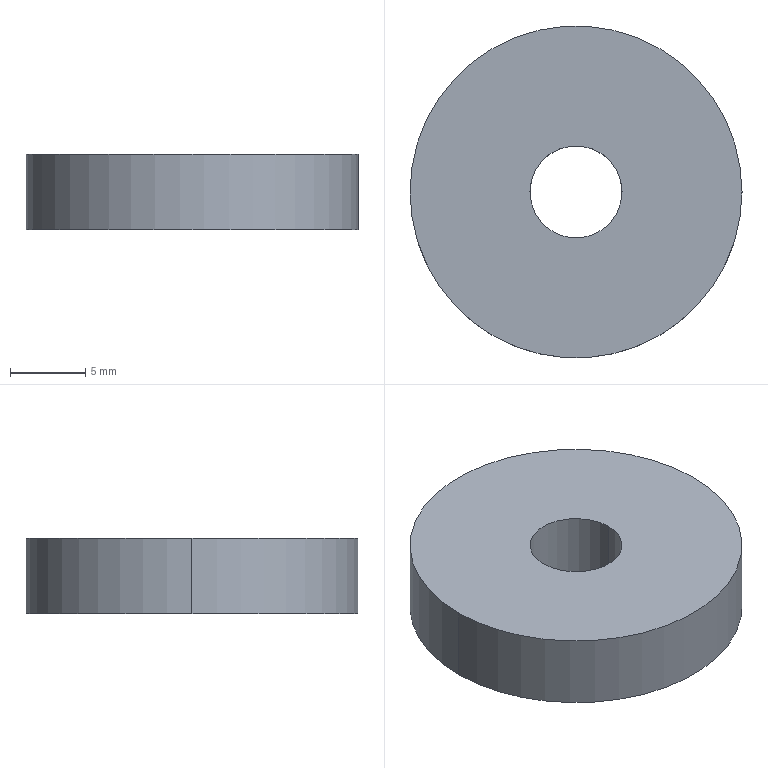Part | NX | features BREP 1 | 1 solid | 6 faces | box 22 x 22 x 5 mm | volume 1755 mm3 | cylinder 4 | plane 2 | commonest cylinder face diameters 6.1 x2 22 x2
STEP:
#1=CARTESIAN_POINT('',(3.05,0.,5.));
#2=VERTEX_POINT('',#1);
#3=CARTESIAN_POINT('',(3.05,0.,0.));
#4=VERTEX_POINT('',#3);
#5=CARTESIAN_POINT('',(3.05,0.,5.));
#6=DIRECTION('',(0.,0.,-1.));
#7=VECTOR('',#6,1000.);
#8=LINE('',#5,#7);
#9=EDGE_CURVE('',#2,#4,#8,.T.);
#10=ORIENTED_EDGE('',*,*,#9,.F.);
#11=CARTESIAN_POINT('',(-3.05,0.,5.));
#12=VERTEX_POINT('',#11);
#13=CARTESIAN_POINT('',(0.,0.,5.));
#14=DIRECTION('',(0.,0.,1.));
#15=DIRECTION('',(1.,0.,0.));
#16=AXIS2_PLACEMENT_3D('',#13,#14,#15);
#17=CIRCLE('',#16,3.05);
#18=EDGE_CURVE('',#2,#12,#17,.T.);
#19=ORIENTED_EDGE('',*,*,#18,.T.);
#20=CARTESIAN_POINT('',(-3.05,0.,0.));
#21=VERTEX_POINT('',#20);
#22=CARTESIAN_POINT('',(-3.05,0.,5.));
#23=DIRECTION('',(0.,0.,-1.));
#24=VECTOR('',#23,1000.);
#25=LINE('',#22,#24);
#26=EDGE_CURVE('',#12,#21,#25,.T.);
#27=ORIENTED_EDGE('',*,*,#26,.T.);
#28=CARTESIAN_POINT('',(0.,0.,0.));
#29=DIRECTION('',(0.,0.,1.));
#30=DIRECTION('',(1.,0.,0.));
#31=AXIS2_PLACEMENT_3D('',#28,#29,#30);
#32=CIRCLE('',#31,3.05);
#33=EDGE_CURVE('',#4,#21,#32,.T.);
#34=ORIENTED_EDGE('',*,*,#33,.F.);
#35=EDGE_LOOP('',(#10,#19,#27,#34));
#36=FACE_BOUND('',#35,.T.);
#37=CARTESIAN_POINT('',(0.,0.,5.));
#38=DIRECTION('',(0.,0.,-1.));
#39=DIRECTION('',(-1.,0.,0.));
#40=AXIS2_PLACEMENT_3D('',#37,#38,#39);
#41=CYLINDRICAL_SURFACE('',#40,3.05);
#42=ADVANCED_FACE('',(#36),#41,.F.);
#43=CARTESIAN_POINT('',(11.,0.,5.));
#44=VERTEX_POINT('',#43);
#45=CARTESIAN_POINT('',(11.,0.,0.));
#46=VERTEX_POINT('',#45);
#47=CARTESIAN_POINT('',(11.,0.,5.));
#48=DIRECTION('',(0.,0.,-1.));
#49=VECTOR('',#48,1000.);
#50=LINE('',#47,#49);
#51=EDGE_CURVE('',#44,#46,#50,.T.);
#52=ORIENTED_EDGE('',*,*,#51,.F.);
#53=CARTESIAN_POINT('',(-11.,0.,5.));
#54=VERTEX_POINT('',#53);
#55=CARTESIAN_POINT('',(0.,0.,5.));
#56=DIRECTION('',(0.,0.,1.));
#57=DIRECTION('',(1.,0.,0.));
#58=AXIS2_PLACEMENT_3D('',#55,#56,#57);
#59=CIRCLE('',#58,11.);
#60=EDGE_CURVE('',#54,#44,#59,.T.);
#61=ORIENTED_EDGE('',*,*,#60,.F.);
#62=CARTESIAN_POINT('',(-11.,0.,0.));
#63=VERTEX_POINT('',#62);
#64=CARTESIAN_POINT('',(-11.,0.,5.));
#65=DIRECTION('',(0.,0.,-1.));
#66=VECTOR('',#65,1000.);
#67=LINE('',#64,#66);
#68=EDGE_CURVE('',#54,#63,#67,.T.);
#69=ORIENTED_EDGE('',*,*,#68,.T.);
#70=CARTESIAN_POINT('',(0.,0.,0.));
#71=DIRECTION('',(0.,0.,1.));
#72=DIRECTION('',(1.,0.,0.));
#73=AXIS2_PLACEMENT_3D('',#70,#71,#72);
#74=CIRCLE('',#73,11.);
#75=EDGE_CURVE('',#63,#46,#74,.T.);
#76=ORIENTED_EDGE('',*,*,#75,.T.);
#77=EDGE_LOOP('',(#52,#61,#69,#76));
#78=FACE_BOUND('',#77,.T.);
#79=CARTESIAN_POINT('',(0.,0.,5.));
#80=DIRECTION('',(0.,0.,-1.));
#81=DIRECTION('',(-1.,0.,0.));
#82=AXIS2_PLACEMENT_3D('',#79,#80,#81);
#83=CYLINDRICAL_SURFACE('',#82,11.);
#84=ADVANCED_FACE('',(#78),#83,.T.);
#85=CARTESIAN_POINT('',(0.,0.,0.));
#86=DIRECTION('',(0.,0.,1.));
#87=DIRECTION('',(1.,0.,0.));
#88=AXIS2_PLACEMENT_3D('',#85,#86,#87);
#89=CIRCLE('',#88,3.05);
#90=EDGE_CURVE('',#21,#4,#89,.T.);
#91=ORIENTED_EDGE('',*,*,#90,.T.);
#92=ORIENTED_EDGE('',*,*,#33,.T.);
#93=EDGE_LOOP('',(#91,#92));
#94=FACE_BOUND('',#93,.T.);
#95=ORIENTED_EDGE('',*,*,#75,.F.);
#96=CARTESIAN_POINT('',(0.,0.,0.));
#97=DIRECTION('',(0.,0.,1.));
#98=DIRECTION('',(1.,0.,0.));
#99=AXIS2_PLACEMENT_3D('',#96,#97,#98);
#100=CIRCLE('',#99,11.);
#101=EDGE_CURVE('',#46,#63,#100,.T.);
#102=ORIENTED_EDGE('',*,*,#101,.F.);
#103=EDGE_LOOP('',(#95,#102));
#104=FACE_BOUND('',#103,.T.);
#105=CARTESIAN_POINT('',(0.,0.,0.));
#106=DIRECTION('',(0.,0.,1.));
#107=DIRECTION('',(1.,0.,0.));
#108=AXIS2_PLACEMENT_3D('',#105,#106,#107);
#109=PLANE('',#108);
#110=ADVANCED_FACE('',(#94,#104),#109,.F.);
#111=CARTESIAN_POINT('',(0.,0.,5.));
#112=DIRECTION('',(0.,0.,1.));
#113=DIRECTION('',(1.,0.,0.));
#114=AXIS2_PLACEMENT_3D('',#111,#112,#113);
#115=CIRCLE('',#114,3.05);
#116=EDGE_CURVE('',#12,#2,#115,.T.);
#117=ORIENTED_EDGE('',*,*,#116,.F.);
#118=ORIENTED_EDGE('',*,*,#18,.F.);
#119=EDGE_LOOP('',(#117,#118));
#120=FACE_BOUND('',#119,.T.);
#121=ORIENTED_EDGE('',*,*,#60,.T.);
#122=CARTESIAN_POINT('',(0.,0.,5.));
#123=DIRECTION('',(0.,0.,1.));
#124=DIRECTION('',(1.,0.,0.));
#125=AXIS2_PLACEMENT_3D('',#122,#123,#124);
#126=CIRCLE('',#125,11.);
#127=EDGE_CURVE('',#44,#54,#126,.T.);
#128=ORIENTED_EDGE('',*,*,#127,.T.);
#129=EDGE_LOOP('',(#121,#128));
#130=FACE_BOUND('',#129,.T.);
#131=CARTESIAN_POINT('',(0.,0.,5.));
#132=DIRECTION('',(0.,0.,1.));
#133=DIRECTION('',(1.,0.,0.));
#134=AXIS2_PLACEMENT_3D('',#131,#132,#133);
#135=PLANE('',#134);
#136=ADVANCED_FACE('',(#120,#130),#135,.T.);
#137=ORIENTED_EDGE('',*,*,#127,.F.);
#138=ORIENTED_EDGE('',*,*,#51,.T.);
#139=ORIENTED_EDGE('',*,*,#101,.T.);
#140=ORIENTED_EDGE('',*,*,#68,.F.);
#141=EDGE_LOOP('',(#137,#138,#139,#140));
#142=FACE_BOUND('',#141,.T.);
#143=CARTESIAN_POINT('',(0.,0.,5.));
#144=DIRECTION('',(0.,0.,-1.));
#145=DIRECTION('',(-1.,0.,0.));
#146=AXIS2_PLACEMENT_3D('',#143,#144,#145);
#147=CYLINDRICAL_SURFACE('',#146,11.);
#148=ADVANCED_FACE('',(#142),#147,.T.);
#149=ORIENTED_EDGE('',*,*,#116,.T.);
#150=ORIENTED_EDGE('',*,*,#9,.T.);
#151=ORIENTED_EDGE('',*,*,#90,.F.);
#152=ORIENTED_EDGE('',*,*,#26,.F.);
#153=EDGE_LOOP('',(#149,#150,#151,#152));
#154=FACE_BOUND('',#153,.T.);
#155=CARTESIAN_POINT('',(0.,0.,5.));
#156=DIRECTION('',(0.,0.,-1.));
#157=DIRECTION('',(-1.,0.,0.));
#158=AXIS2_PLACEMENT_3D('',#155,#156,#157);
#159=CYLINDRICAL_SURFACE('',#158,3.05);
#160=ADVANCED_FACE('',(#154),#159,.F.);
#161=CLOSED_SHELL('',(#42,#84,#110,#136,#148,#160));
#162=MANIFOLD_SOLID_BREP('',#161);
#163=(LENGTH_UNIT()NAMED_UNIT(*)SI_UNIT(.MILLI.,.METRE.));
#164=UNCERTAINTY_MEASURE_WITH_UNIT(LENGTH_MEASURE(0.00001),#163,'','');
#165=(NAMED_UNIT(*)PLANE_ANGLE_UNIT()SI_UNIT($,.RADIAN.));
#166=(NAMED_UNIT(*)SI_UNIT($,.STERADIAN.)SOLID_ANGLE_UNIT());
#167=(GEOMETRIC_REPRESENTATION_CONTEXT(3)GLOBAL_UNCERTAINTY_ASSIGNED_CONTEXT((#164))GLOBAL_UNIT_ASSIGNED_CONTEXT((#163,#165,#166))REPRESENTATION_CONTEXT('',''));
#168=ADVANCED_BREP_SHAPE_REPRESENTATION('',(#162),#167);